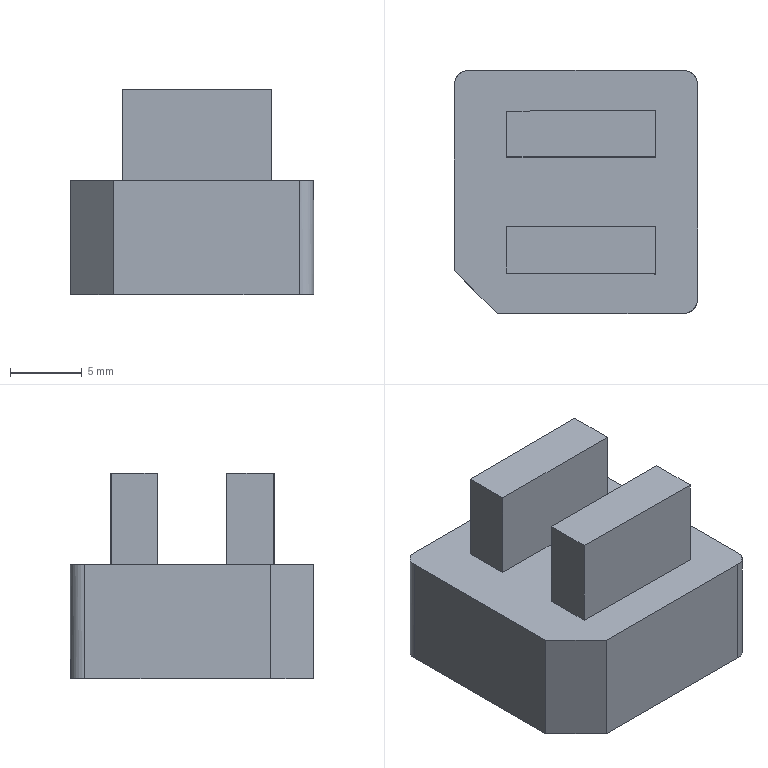NC program | PowerMill | posted with a generic post | part box 17 x 17 x 14.396 mm
Lines 7229 to 8093 of 69084:
N7326 M6
N7327 S18000 M03
N7328 G00 G90 X0.0 Y0.0
N7329 G43 Z10.796 H10
N7330
N7331 G05 P10000 R8
N7332 X6.5722 Y-7.4268
N7333 Z0.918
N7334 G01 Z-0.282 F1200.0
N7335 X6.5582 Y-7.3853 F2000.0
N7336 X6.5405 Y-7.3453
N7337 X6.5192 Y-7.3071
N7338 X6.4946 Y-7.2709
N7339 X6.4667 Y-7.2372
N7340 X6.4359 Y-7.2061
N7341 X6.4024 Y-7.178
N7342 X6.3664 Y-7.153
N7343 X6.3284 Y-7.1314
N7344 X6.2885 Y-7.1134
N7345 X6.2472 Y-7.0991
N7346 X6.2047 Y-7.0886
N7347 X6.1614 Y-7.082
N7348 X6.1178 Y-7.0793
N7349 X6.074 Y-7.0807
N7350 X6.0306 Y-7.086
N7351 X5.9879 Y-7.0953
N7352 X5.9783 Y-7.0979
N7353 X5.9106 Y-7.1174
N7354 X5.8358 Y-7.1349
N7355 X5.7731 Y-7.1469
N7356 X5.7091 Y-7.1555
N7357 X5.6389 Y-7.1612
N7358 X5.5591 Y-7.1639
N7359 X5.4625
N7360 X3.8431 Y-7.1555
N7361 X2.0292 Y-7.1459
N7362 X-1.5322 Y-7.1273
N7363 X-3.5989 Y-7.1165
N7364 X-4.5402 Y-7.1116
N7365 X-4.8986 Y-7.109
N7366 X-4.972 Y-7.1064
N7367 X-5.0454 Y-7.0998
N7368 X-5.1187 Y-7.0892
N7369 X-5.1917 Y-7.0746
N7370 X-5.2643 Y-7.0561
N7371 X-5.3362 Y-7.0336
N7372 X-5.4072 Y-7.0072
N7373 X-5.4764 Y-6.9773
N7374 X-5.544 Y-6.9437
N7375 X-5.6097 Y-6.9066
N7376 X-5.6733 Y-6.866
N7377 X-5.7347 Y-6.8222
N7378 X-5.7937 Y-6.7752
N7379 X-5.8502 Y-6.7251
N7380 X-5.9039 Y-6.6721
N7381 X-5.9547 Y-6.6163
N7382 X-6.0024 Y-6.5579
N7383 X-6.0471 Y-6.4971
N7384 X-6.0884 Y-6.434
N7385 X-6.1264 Y-6.3688
N7386 X-6.1608 Y-6.3016
N7387 X-6.1916 Y-6.2329
N7388 X-6.219 Y-6.1623
N7389 X-6.2424 Y-6.0908
N7390 X-6.2619 Y-6.0185
N7391 X-6.2774 Y-5.9457
N7392 X-6.289 Y-5.8725
N7393 X-6.2966 Y-5.7992
N7394 X-6.3002 Y-5.7258
N7395 X-6.3005 Y-5.6523
N7396 X-6.3012 Y-4.2054
N7397 Y-3.3524
N7398 X-6.3017 Y-2.6994
N7399 X-6.3024 Y-2.4993
N7400 X-6.3011 Y-2.4058
N7401 X-6.2965 Y-2.3214
N7402 X-6.2887 Y-2.2438
N7403 X-6.2779 Y-2.1715
N7404 X-6.264 Y-2.1038
N7405 X-6.2465 Y-2.0368
N7406 X-6.2239 Y-1.9652
N7407 X-6.1974 Y-1.8947
N7408 X-6.1672 Y-1.8256
N7409 X-6.1333 Y-1.758
N7410 X-6.0959 Y-1.6922
N7411 X-6.0549 Y-1.6284
N7412 X-6.0109 Y-1.5671
N7413 X-5.9638 Y-1.5084
N7414 X-5.9137 Y-1.4522
N7415 X-5.8606 Y-1.3987
N7416 X-5.8048 Y-1.3481
N7417 X-5.7463 Y-1.3005
N7418 X-5.6855 Y-1.2561
N7419 X-5.6224 Y-1.215
N7420 X-5.5572 Y-1.1773
N7421 X-5.4901 Y-1.1432
N7422 X-5.4214 Y-1.1126
N7423 X-5.3656 Y-1.0909
N7424 X-5.31 Y-1.0716
N7425 X-5.2537 Y-1.0546
N7426 X-5.1954 Y-1.0398
N7427 X-5.134 Y-1.0273
N7428 X-5.0677 Y-1.0172
N7429 X-4.9943 Y-1.0097
N7430 X-4.9128 Y-1.0052
N7431 X-4.8359 Y-1.0034
N7432 X-4.7635 Y-1.0031
N7433 X-4.6941 Y-1.0033
N7434 X-4.6232 Y-1.0036
N7435 X-4.0059 Y-1.0045
N7436 X-3.399 Y-1.0041
N7437 X3.1113
N7438 X4.6304 Y-1.0037
N7439 X5.4985 Y-1.0031
N7440 X5.5826 Y-1.0047
N7441 X5.6636 Y-1.0098
N7442 X5.7417 Y-1.0183
N7443 X5.8171 Y-1.0304
N7444 X5.8901 Y-1.046
N7445 X5.9609 Y-1.0651
N7446 X6.0297 Y-1.0877
N7447 X6.0967 Y-1.1137
N7448 X6.1625 Y-1.1433
N7449 X6.23 Y-1.1779
N7450 X6.2955 Y-1.2159
N7451 X6.3588 Y-1.2573
N7452 X6.4199 Y-1.302
N7453 X6.4785 Y-1.3499
N7454 X6.5334 Y-1.3996
N7455 X6.5866 Y-1.4532
N7456 X6.6367 Y-1.5093
N7457 X6.6836 Y-1.5678
N7458 X6.727 Y-1.6283
N7459 X6.767 Y-1.6908
N7460 X6.8034 Y-1.7551
N7461 X6.8362 Y-1.821
N7462 X6.8679 Y-1.8929
N7463 X6.8946 Y-1.9626
N7464 X6.9166 Y-2.0305
N7465 X6.9341 Y-2.0969
N7466 X6.9464 Y-2.1543
N7467 X6.9565 Y-2.212
N7468 X6.9642 Y-2.2701
N7469 X6.9696 Y-2.3309
N7470 X6.9729 Y-2.4057
N7471 X6.9738 Y-2.4747
N7472 X6.9737 Y-2.5336
N7473 X6.9735 Y-2.5924
N7474 X6.9734 Y-2.6511
N7475 X6.9731 Y-3.8243
N7476 X6.973 Y-5.0696
N7477 X6.9739 Y-5.6984
N7478 X6.9723 Y-5.7835
N7479 X6.967 Y-5.8646
N7480 X6.9582 Y-5.942
N7481 X6.946 Y-6.0161
N7482 X6.9304 Y-6.0871
N7483 X6.9116 Y-6.1553
N7484 X6.8892 Y-6.2216
N7485 X6.8608 Y-6.2937
N7486 X6.8291 Y-6.3634
N7487 X6.7942 Y-6.4306
N7488 X6.7562 Y-6.4953
N7489 X6.7152 Y-6.5573
N7490 X6.671 Y-6.6169
N7491 X6.623 Y-6.6751
N7492 X6.5719 Y-6.7306
N7493 X6.518 Y-6.7834
N7494 X6.4613 Y-6.8333
N7495 X6.4021 Y-6.8802
N7496 X6.3405 Y-6.9238
N7497 X6.2767 Y-6.9641
N7498 X6.2109 Y-7.0009
N7499 X6.1433 Y-7.0342
N7500 X6.074 Y-7.0639
N7501 X6.0032 Y-7.0898
N7502 X5.9783 Y-7.0979
N7503 X5.9211 Y-7.114
N7504 X5.8523 Y-7.1314 Z-0.2821
N7505 X5.794 Y-7.143
N7506 X5.7224 Y-7.1532 Z-0.2822
N7507 X5.6471 Y-7.1601
N7508 X5.5652 Y-7.1636 Z-0.2823
N7509 X5.4742 Y-7.164 Z-0.2824
N7510 X3.8613 Y-7.1556 Z-0.2837
N7511 X2.0473 Y-7.146 Z-0.2852
N7512 X-1.5144 Y-7.1274 Z-0.2881
N7513 X-3.5989 Y-7.1165 Z-0.2898
N7514 X-4.5388 Y-7.1116 Z-0.2906
N7515 X-4.8986 Y-7.109 Z-0.2909
N7516 X-4.972 Y-7.1064 Z-0.291
N7517 X-5.0454 Y-7.0998
N7518 X-5.1187 Y-7.0892 Z-0.2911
N7519 X-5.1917 Y-7.0746 Z-0.2912
N7520 X-5.2643 Y-7.0561
N7521 X-5.3362 Y-7.0336 Z-0.2913
N7522 X-5.4073 Y-7.0072
N7523 X-5.4764 Y-6.9773 Z-0.2914
N7524 X-5.544 Y-6.9437 Z-0.2915
N7525 X-5.6097 Y-6.9066
N7526 X-5.6734 Y-6.866 Z-0.2916
N7527 X-5.7348 Y-6.8222 Z-0.2917
N7528 X-5.7938 Y-6.7751
N7529 X-5.8502 Y-6.725 Z-0.2918
N7530 X-5.9039 Y-6.672
N7531 X-5.9547 Y-6.6163 Z-0.2919
N7532 X-6.0025 Y-6.5579 Z-0.292
N7533 X-6.0471 Y-6.497
N7534 X-6.0885 Y-6.4339 Z-0.2921
N7535 X-6.1264 Y-6.3687 Z-0.2922
N7536 X-6.1609 Y-6.3016
N7537 X-6.1917 Y-6.2329 Z-0.2923
N7538 X-6.219 Y-6.1623
N7539 X-6.2424 Y-6.0907 Z-0.2924
N7540 X-6.2619 Y-6.0185 Z-0.2925
N7541 X-6.2775 Y-5.9456
N7542 X-6.289 Y-5.8724 Z-0.2926
N7543 X-6.2966 Y-5.7991
N7544 X-6.3002 Y-5.7258 Z-0.2927
N7545 X-6.3005 Y-5.6523 Z-0.2928
N7546 X-6.3012 Y-4.1928 Z-0.294
N7547 Y-3.3325 Z-0.2947
N7548 X-6.3018 Y-2.6011 Z-0.2953
N7549 X-6.3022 Y-2.4722 Z-0.2954
N7550 X-6.301 Y-2.3964
N7551 X-6.2967 Y-2.3205 Z-0.2955
N7552 X-6.2889 Y-2.2449 Z-0.2956
N7553 X-6.2774 Y-2.1708
N7554 X-6.2623 Y-2.099 Z-0.2957
N7555 X-6.2439 Y-2.0295 Z-0.2958
N7556 X-6.2221 Y-1.9608
N7557 X-6.1958 Y-1.891 Z-0.2959
N7558 X-6.1657 Y-1.8224
N7559 X-6.132 Y-1.7554 Z-0.296
N7560 X-6.0946 Y-1.6901 Z-0.2961
N7561 X-6.0537 Y-1.6266
N7562 X-6.0093 Y-1.5652 Z-0.2962
N7563 X-5.9617 Y-1.506
N7564 X-5.9114 Y-1.4499 Z-0.2963
N7565 X-5.8582 Y-1.3965 Z-0.2964
N7566 X-5.8022 Y-1.346
N7567 X-5.7437 Y-1.2985 Z-0.2965
N7568 X-5.6827 Y-1.2542 Z-0.2966
N7569 X-5.6195 Y-1.2133
N7570 X-5.5543 Y-1.1757 Z-0.2967
N7571 X-5.4865 Y-1.1413
N7572 X-5.4174 Y-1.1106 Z-0.2968
N7573 X-5.3472 Y-1.0837 Z-0.2969
N7574 X-5.276 Y-1.0608
N7575 X-5.2042 Y-1.0418 Z-0.297
N7576 X-5.132 Y-1.0268
N7577 X-5.0594 Y-1.0157 Z-0.2971
N7578 X-4.9868 Y-1.0087 Z-0.2972
N7579 X-4.9142 Y-1.0056
N7580 X-4.8415 Y-1.0053 Z-0.2973
N7581 X-3.8933 Y-1.0042 Z-0.2981
N7582 X-2.316 Y-1.0041 Z-0.2994
N7583 X3.5448 Y-1.0039 Z-0.3042
N7584 X5.2855 Y-1.0033 Z-0.3056
N7585 X5.4985 Y-1.003 Z-0.3058
N7586 X5.5827 Y-1.0046 Z-0.3059
N7587 X5.6637 Y-1.0097
N7588 X5.7419 Y-1.0183 Z-0.306
N7589 X5.8173 Y-1.0304 Z-0.3061
N7590 X5.8903 Y-1.046
N7591 X5.961 Y-1.0651 Z-0.3062
N7592 X6.0297 Y-1.0876
N7593 X6.0966 Y-1.1136 Z-0.3063
N7594 X6.1624 Y-1.1432 Z-0.3064
N7595 X6.2299 Y-1.1778
N7596 X6.2954 Y-1.2158 Z-0.3065
N7597 X6.3588 Y-1.2573 Z-0.3066
N7598 X6.4198 Y-1.3019
N7599 X6.4783 Y-1.3497 Z-0.3067
N7600 X6.5343 Y-1.4006
N7601 X6.5874 Y-1.4543 Z-0.3068
N7602 X6.6375 Y-1.5104 Z-0.3069
N7603 X6.6845 Y-1.5692
N7604 X6.7283 Y-1.6304 Z-0.307
N7605 X6.7689 Y-1.6939 Z-0.3071
N7606 X6.8061 Y-1.7595
N7607 X6.8397 Y-1.827 Z-0.3072
N7608 X6.8698 Y-1.8962
N7609 X6.8964 Y-1.967 Z-0.3073
N7610 X6.9188 Y-2.0366 Z-0.3074
N7611 X6.9364 Y-2.1032
N7612 X6.9495 Y-2.1672 Z-0.3075
N7613 X6.9552 Y-2.204
N7614 X6.9606 Y-2.2409
N7615 X6.9661 Y-2.2778 Z-0.3076
N7616 X6.9703 Y-2.3149
N7617 X6.9722 Y-2.3521
N7618 X6.9728 Y-2.3893 Z-0.3077
N7619 X6.9729 Y-2.4266
N7620 X6.9732 Y-2.8429 Z-0.308
N7621 X6.9733 Y-4.3499 Z-0.3093
N7622 X6.9741 Y-5.6983 Z-0.3104
N7623 X6.9724 Y-5.7818
N7624 X6.9671 Y-5.8623 Z-0.3105
N7625 X6.9582 Y-5.94 Z-0.3106
N7626 X6.9457 Y-6.0153
N7627 X6.9297 Y-6.0882 Z-0.3107
N7628 X6.9102 Y-6.1589 Z-0.3108
N7629 X6.8872 Y-6.2277
N7630 X6.8607 Y-6.2947 Z-0.3109
N7631 X6.8306 Y-6.3606
N7632 X6.7956 Y-6.4281 Z-0.311
N7633 X6.7571 Y-6.4935 Z-0.3111
N7634 X6.7154 Y-6.5567
N7635 X6.6704 Y-6.6174 Z-0.3112
N7636 X6.6224 Y-6.6756 Z-0.3113
N7637 X6.5714 Y-6.7311
N7638 X6.5176 Y-6.7839 Z-0.3114
N7639 X6.461 Y-6.8337
N7640 X6.4018 Y-6.8804 Z-0.3115
N7641 X6.3403 Y-6.924 Z-0.3116
N7642 X6.2765 Y-6.9643
N7643 X6.2106 Y-7.0011 Z-0.3117
N7644 X6.143 Y-7.0343 Z-0.3118
N7645 X6.0737 Y-7.064
N7646 X6.0029 Y-7.0899 Z-0.3119
N7647 X5.9783 Y-7.0979
N7648 X5.9211 Y-7.114
N7649 X5.8523 Y-7.1314 Z-0.312
N7650 X5.794 Y-7.143 Z-0.3121
N7651 X5.7224 Y-7.1532
N7652 X5.6471 Y-7.1601 Z-0.3122
N7653 X5.5652 Y-7.1636
N7654 X5.4742 Y-7.164 Z-0.3123
N7655 X3.8613 Y-7.1556 Z-0.3136
N7656 X2.0473 Y-7.146 Z-0.3151
N7657 X-1.5144 Y-7.1274 Z-0.3181
N7658 X-3.5989 Y-7.1165 Z-0.3198
N7659 X-4.5388 Y-7.1116 Z-0.3206
N7660 X-4.8986 Y-7.109 Z-0.3209
N7661 X-4.972 Y-7.1064
N7662 X-5.0454 Y-7.0998 Z-0.321
N7663 X-5.1187 Y-7.0892
N7664 X-5.1917 Y-7.0746 Z-0.3211
N7665 X-5.2643 Y-7.0561 Z-0.3212
N7666 X-5.3362 Y-7.0336
N7667 X-5.4073 Y-7.0072 Z-0.3213
N7668 X-5.4764 Y-6.9773
N7669 X-5.544 Y-6.9437 Z-0.3214
N7670 X-5.6097 Y-6.9066 Z-0.3215
N7671 X-5.6734 Y-6.866
N7672 X-5.7348 Y-6.8222 Z-0.3216
N7673 X-5.7938 Y-6.7751 Z-0.3217
N7674 X-5.8502 Y-6.725
N7675 X-5.9039 Y-6.672 Z-0.3218
N7676 X-5.9547 Y-6.6163
N7677 X-6.0025 Y-6.5579 Z-0.3219
N7678 X-6.0471 Y-6.497 Z-0.322
N7679 X-6.0885 Y-6.4339
N7680 X-6.1264 Y-6.3687 Z-0.3221
N7681 X-6.1609 Y-6.3016 Z-0.3222
N7682 X-6.1917 Y-6.2329
N7683 X-6.219 Y-6.1623 Z-0.3223
N7684 X-6.2424 Y-6.0907
N7685 X-6.2619 Y-6.0185 Z-0.3224
N7686 X-6.2775 Y-5.9456 Z-0.3225
N7687 X-6.289 Y-5.8724
N7688 X-6.2966 Y-5.7991 Z-0.3226
N7689 X-6.3002 Y-5.7258
N7690 X-6.3005 Y-5.6523 Z-0.3227
N7691 X-6.3012 Y-4.1928 Z-0.3239
N7692 Y-3.3325 Z-0.3246
N7693 X-6.3018 Y-2.6011 Z-0.3252
N7694 X-6.3022 Y-2.4722 Z-0.3253
N7695 X-6.301 Y-2.3964 Z-0.3254
N7696 X-6.2967 Y-2.3205 Z-0.3255
N7697 X-6.2889 Y-2.2449
N7698 X-6.2774 Y-2.1708 Z-0.3256
N7699 X-6.2623 Y-2.099
N7700 X-6.2439 Y-2.0295 Z-0.3257
N7701 X-6.2221 Y-1.9608 Z-0.3258
N7702 X-6.1958 Y-1.891
N7703 X-6.1657 Y-1.8224 Z-0.3259
N7704 X-6.132 Y-1.7554
N7705 X-6.0946 Y-1.6901 Z-0.326
N7706 X-6.0537 Y-1.6266 Z-0.3261
N7707 X-6.0093 Y-1.5652
N7708 X-5.9617 Y-1.506 Z-0.3262
N7709 X-5.9114 Y-1.4499
N7710 X-5.8582 Y-1.3965 Z-0.3263
N7711 X-5.8022 Y-1.346 Z-0.3264
N7712 X-5.7437 Y-1.2985
N7713 X-5.6827 Y-1.2542 Z-0.3265
N7714 X-5.6195 Y-1.2133 Z-0.3266
N7715 X-5.5543 Y-1.1757
N7716 X-5.4865 Y-1.1413 Z-0.3267
N7717 X-5.4174 Y-1.1106
N7718 X-5.3472 Y-1.0837 Z-0.3268
N7719 X-5.276 Y-1.0608 Z-0.3269
N7720 X-5.2042 Y-1.0418
N7721 X-5.132 Y-1.0268 Z-0.327
N7722 X-5.0594 Y-1.0157 Z-0.3271
N7723 X-4.9868 Y-1.0087
N7724 X-4.9142 Y-1.0056 Z-0.3272
N7725 X-4.8415 Y-1.0053
N7726 X-3.8933 Y-1.0042 Z-0.328
N7727 X-2.316 Y-1.0041 Z-0.3293
N7728 X3.5448 Y-1.0039 Z-0.3341
N7729 X5.2855 Y-1.0033 Z-0.3356
N7730 X5.4985 Y-1.003 Z-0.3357
N7731 X5.5827 Y-1.0046 Z-0.3358
N7732 X5.6637 Y-1.0097 Z-0.3359
N7733 X5.7419 Y-1.0183
N7734 X5.8173 Y-1.0304 Z-0.336
N7735 X5.8903 Y-1.046 Z-0.3361
N7736 X5.961 Y-1.0651
N7737 X6.0297 Y-1.0876 Z-0.3362
N7738 X6.0966 Y-1.1136
N7739 X6.1624 Y-1.1432 Z-0.3363
N7740 X6.2299 Y-1.1778 Z-0.3364
N7741 X6.2954 Y-1.2158
N7742 X6.3588 Y-1.2573 Z-0.3365
N7743 X6.4198 Y-1.3019 Z-0.3366
N7744 X6.4783 Y-1.3497
N7745 X6.5343 Y-1.4006 Z-0.3367
N7746 X6.5874 Y-1.4543
N7747 X6.6375 Y-1.5104 Z-0.3368
N7748 X6.6845 Y-1.5692 Z-0.3369
N7749 X6.7283 Y-1.6304
N7750 X6.7689 Y-1.6939 Z-0.337
N7751 X6.8061 Y-1.7595 Z-0.3371
N7752 X6.8397 Y-1.827
N7753 X6.8698 Y-1.8962 Z-0.3372
N7754 X6.8964 Y-1.967
N7755 X6.9188 Y-2.0366 Z-0.3373
N7756 X6.9364 Y-2.1032 Z-0.3374
N7757 X6.9495 Y-2.1672
N7758 X6.9552 Y-2.204
N7759 X6.9606 Y-2.2409 Z-0.3375
N7760 X6.9661 Y-2.2778
N7761 X6.9703 Y-2.3149
N7762 X6.9722 Y-2.3521 Z-0.3376
N7763 X6.9728 Y-2.3893
N7764 X6.9729 Y-2.4266
N7765 X6.9732 Y-2.8429 Z-0.338
N7766 X6.9733 Y-4.3499 Z-0.3392
N7767 X6.9741 Y-5.6983 Z-0.3403
N7768 X6.9724 Y-5.7818 Z-0.3404
N7769 X6.9671 Y-5.8623 Z-0.3405
N7770 X6.9582 Y-5.94
N7771 X6.9457 Y-6.0153 Z-0.3406
N7772 X6.9297 Y-6.0882
N7773 X6.9102 Y-6.1589 Z-0.3407
N7774 X6.8872 Y-6.2277 Z-0.3408
N7775 X6.8607 Y-6.2947
N7776 X6.8306 Y-6.3606 Z-0.3409
N7777 X6.7956 Y-6.4281
N7778 X6.7571 Y-6.4935 Z-0.341
N7779 X6.7154 Y-6.5567 Z-0.3411
N7780 X6.6704 Y-6.6174
N7781 X6.6224 Y-6.6756 Z-0.3412
N7782 X6.5714 Y-6.7311 Z-0.3413
N7783 X6.5176 Y-6.7839
N7784 X6.461 Y-6.8337 Z-0.3414
N7785 X6.4018 Y-6.8804
N7786 X6.3403 Y-6.924 Z-0.3415
N7787 X6.2765 Y-6.9643 Z-0.3416
N7788 X6.2106 Y-7.0011
N7789 X6.143 Y-7.0343 Z-0.3417
N7790 X6.0737 Y-7.064 Z-0.3418
N7791 X6.0029 Y-7.0899
N7792 X5.9783 Y-7.0979
N7793 X5.9211 Y-7.114 Z-0.3419
N7794 X5.8523 Y-7.1314
N7795 X5.794 Y-7.143 Z-0.342
N7796 X5.7224 Y-7.1532 Z-0.3421
N7797 X5.6471 Y-7.1601
N7798 X5.5652 Y-7.1636 Z-0.3422
N7799 X5.4742 Y-7.164 Z-0.3423
N7800 X3.8613 Y-7.1556 Z-0.3436
N7801 X2.0473 Y-7.146 Z-0.3451
N7802 X-1.5144 Y-7.1274 Z-0.348
N7803 X-3.5989 Y-7.1165 Z-0.3497
N7804 X-4.5388 Y-7.1116 Z-0.3505
N7805 X-4.8986 Y-7.109 Z-0.3508
N7806 X-4.972 Y-7.1064 Z-0.3509
N7807 X-5.0454 Y-7.0998
N7808 X-5.1187 Y-7.0892 Z-0.351
N7809 X-5.1917 Y-7.0746
N7810 X-5.2643 Y-7.0561 Z-0.3511
N7811 X-5.3362 Y-7.0336 Z-0.3512
N7812 X-5.4073 Y-7.0072
N7813 X-5.4764 Y-6.9773 Z-0.3513
N7814 X-5.544 Y-6.9437 Z-0.3514
N7815 X-5.6097 Y-6.9066
N7816 X-5.6734 Y-6.866 Z-0.3515
N7817 X-5.7348 Y-6.8222
N7818 X-5.7938 Y-6.7751 Z-0.3516
N7819 X-5.8502 Y-6.725 Z-0.3517
N7820 X-5.9039 Y-6.672
N7821 X-5.9547 Y-6.6163 Z-0.3518
N7822 X-6.0025 Y-6.5579
N7823 X-6.0471 Y-6.497 Z-0.3519
N7824 X-6.0885 Y-6.4339 Z-0.352
N7825 X-6.1264 Y-6.3687
N7826 X-6.1609 Y-6.3016 Z-0.3521
N7827 X-6.1917 Y-6.2329 Z-0.3522
N7828 X-6.219 Y-6.1623
N7829 X-6.2424 Y-6.0907 Z-0.3523
N7830 X-6.2619 Y-6.0185
N7831 X-6.2775 Y-5.9456 Z-0.3524
N7832 X-6.289 Y-5.8724 Z-0.3525
N7833 X-6.2966 Y-5.7991
N7834 X-6.3002 Y-5.7258 Z-0.3526
N7835 X-6.3005 Y-5.6523
N7836 X-6.3012 Y-4.1928 Z-0.3539
N7837 Y-3.3325 Z-0.3546
N7838 X-6.3018 Y-2.6011 Z-0.3552
N7839 X-6.3022 Y-2.4722 Z-0.3553
N7840 X-6.301 Y-2.3964
N7841 X-6.2967 Y-2.3205 Z-0.3554
N7842 X-6.2889 Y-2.2449 Z-0.3555
N7843 X-6.2774 Y-2.1708
N7844 X-6.2623 Y-2.099 Z-0.3556
N7845 X-6.2439 Y-2.0295
N7846 X-6.2221 Y-1.9608 Z-0.3557
N7847 X-6.1958 Y-1.891 Z-0.3558
N7848 X-6.1657 Y-1.8224
N7849 X-6.132 Y-1.7554 Z-0.3559
N7850 X-6.0946 Y-1.6901
N7851 X-6.0537 Y-1.6266 Z-0.356
N7852 X-6.0093 Y-1.5652 Z-0.3561
N7853 X-5.9617 Y-1.506
N7854 X-5.9114 Y-1.4499 Z-0.3562
N7855 X-5.8582 Y-1.3965 Z-0.3563
N7856 X-5.8022 Y-1.346
N7857 X-5.7437 Y-1.2985 Z-0.3564
N7858 X-5.6827 Y-1.2542
N7859 X-5.6195 Y-1.2133 Z-0.3565
N7860 X-5.5543 Y-1.1757 Z-0.3566
N7861 X-5.4865 Y-1.1413
N7862 X-5.4174 Y-1.1106 Z-0.3567
N7863 X-5.3472 Y-1.0837 Z-0.3568
N7864 X-5.276 Y-1.0608
N7865 X-5.2042 Y-1.0418 Z-0.3569
N7866 X-5.132 Y-1.0268
N7867 X-5.0594 Y-1.0157 Z-0.357
N7868 X-4.9868 Y-1.0087 Z-0.3571
N7869 X-4.9142 Y-1.0056
N7870 X-4.8415 Y-1.0053 Z-0.3572
N7871 X-3.8933 Y-1.0042 Z-0.358
N7872 X-2.316 Y-1.0041 Z-0.3593
N7873 X3.5448 Y-1.0039 Z-0.3641
N7874 X5.2853 Y-1.0033 Z-0.3655
N7875 X5.4985 Y-1.003 Z-0.3657
N7876 X5.5825 Y-1.0046 Z-0.3658
N7877 X5.6635 Y-1.0097
N7878 X5.7416 Y-1.0182 Z-0.3659
N7879 X5.817 Y-1.0303 Z-0.366
N7880 X5.89 Y-1.0459
N7881 X5.9607 Y-1.065 Z-0.3661
N7882 X6.0295 Y-1.0875
N7883 X6.0964 Y-1.1136 Z-0.3662
N7884 X6.1623 Y-1.1432 Z-0.3663
N7885 X6.2298 Y-1.1777
N7886 X6.2953 Y-1.2158 Z-0.3664
N7887 X6.3586 Y-1.2572
N7888 X6.4197 Y-1.3018 Z-0.3665
N7889 X6.4782 Y-1.3496 Z-0.3666
N7890 X6.5342 Y-1.4005
N7891 X6.5873 Y-1.4542 Z-0.3667
N7892 X6.6374 Y-1.5103
N7893 X6.6844 Y-1.5691 Z-0.3668
N7894 X6.7282 Y-1.6302 Z-0.3669
N7895 X6.7688 Y-1.6937
N7896 X6.806 Y-1.7594 Z-0.367
N7897 X6.8397 Y-1.8269 Z-0.3671
N7898 X6.8697 Y-1.8961
N7899 X6.8964 Y-1.9669 Z-0.3672
N7900 X6.9188 Y-2.0364
N7901 X6.9364 Y-2.103 Z-0.3673
N7902 X6.9494 Y-2.1671 Z-0.3674
N7903 X6.9552 Y-2.2039
N7904 X6.9606 Y-2.2408
N7905 X6.9661 Y-2.2777
N7906 X6.9703 Y-2.3148 Z-0.3675
N7907 X6.9722 Y-2.352
N7908 X6.9728 Y-2.3892
N7909 X6.9729 Y-2.4265 Z-0.3676
N7910 X6.9732 Y-2.8427 Z-0.3679
N7911 X6.9733 Y-4.3498 Z-0.3692
N7912 X6.9741 Y-5.6983 Z-0.3703
N7913 X6.9724 Y-5.7818
N7914 X6.9671 Y-5.8623 Z-0.3704
N7915 X6.9582 Y-5.94 Z-0.3705
N7916 X6.9457 Y-6.0153
N7917 X6.9297 Y-6.0882 Z-0.3706
N7918 X6.9102 Y-6.1589
N7919 X6.8872 Y-6.2277 Z-0.3707
N7920 X6.8607 Y-6.2947 Z-0.3708
N7921 X6.8306 Y-6.3606
N7922 X6.7956 Y-6.4281 Z-0.3709
N7923 X6.7571 Y-6.4935 Z-0.371
N7924 X6.7154 Y-6.5567
N7925 X6.6704 Y-6.6174 Z-0.3711
N7926 X6.6224 Y-6.6756
N7927 X6.5714 Y-6.7311 Z-0.3712
N7928 X6.5176 Y-6.7839 Z-0.3713
N7929 X6.461 Y-6.8337
N7930 X6.4018 Y-6.8804 Z-0.3714
N7931 X6.3403 Y-6.924
N7932 X6.2765 Y-6.9643 Z-0.3715
N7933 X6.2106 Y-7.0011 Z-0.3716
N7934 X6.143 Y-7.0343
N7935 X6.0737 Y-7.064 Z-0.3717
N7936 X6.0029 Y-7.0899 Z-0.3718
N7937 X5.9783 Y-7.0979
N7938 X5.9211 Y-7.114
N7939 X5.8523 Y-7.1314 Z-0.3719
N7940 X5.794 Y-7.143
N7941 X5.7224 Y-7.1532 Z-0.372
N7942 X5.6471 Y-7.1601 Z-0.3721
N7943 X5.5652 Y-7.1636
N7944 X5.4742 Y-7.164 Z-0.3722
N7945 X3.8613 Y-7.1556 Z-0.3735
N7946 X2.0473 Y-7.146 Z-0.375
N7947 X-1.5144 Y-7.1274 Z-0.378
N7948 X-3.5989 Y-7.1165 Z-0.3797
N7949 X-4.5388 Y-7.1116 Z-0.3804
N7950 X-4.8986 Y-7.109 Z-0.3807
N7951 X-4.972 Y-7.1064 Z-0.3808
N7952 X-5.0454 Y-7.0998 Z-0.3809
N7953 X-5.1187 Y-7.0892
N7954 X-5.1917 Y-7.0746 Z-0.381
N7955 X-5.2643 Y-7.0561
N7956 X-5.3362 Y-7.0336 Z-0.3811
N7957 X-5.4073 Y-7.0072 Z-0.3812
N7958 X-5.4764 Y-6.9773
N7959 X-5.544 Y-6.9437 Z-0.3813
N7960 X-5.6097 Y-6.9066 Z-0.3814
N7961 X-5.6734 Y-6.866
N7962 X-5.7348 Y-6.8222 Z-0.3815
N7963 X-5.7938 Y-6.7751
N7964 X-5.8502 Y-6.725 Z-0.3816
N7965 X-5.9039 Y-6.672 Z-0.3817
N7966 X-5.9547 Y-6.6163
N7967 X-6.0025 Y-6.5579 Z-0.3818
N7968 X-6.0471 Y-6.497 Z-0.3819
N7969 X-6.0885 Y-6.4339
N7970 X-6.1264 Y-6.3687 Z-0.382
N7971 X-6.1609 Y-6.3016
N7972 X-6.1917 Y-6.2329 Z-0.3821
N7973 X-6.219 Y-6.1623 Z-0.3822
N7974 X-6.2424 Y-6.0907
N7975 X-6.2619 Y-6.0185 Z-0.3823
N7976 X-6.2775 Y-5.9456
N7977 X-6.289 Y-5.8724 Z-0.3824
N7978 X-6.2966 Y-5.7991 Z-0.3825
N7979 X-6.3002 Y-5.7258
N7980 X-6.3005 Y-5.6523 Z-0.3826
N7981 X-6.3012 Y-4.1928 Z-0.3838
N7982 Y-3.3325 Z-0.3845
N7983 X-6.3018 Y-2.6011 Z-0.3851
N7984 X-6.3022 Y-2.4722 Z-0.3852
N7985 X-6.301 Y-2.3964 Z-0.3853
N7986 X-6.2967 Y-2.3205
N7987 X-6.2889 Y-2.2449 Z-0.3854
N7988 X-6.2774 Y-2.1708 Z-0.3855
N7989 X-6.2623 Y-2.099
N7990 X-6.2439 Y-2.0295 Z-0.3856
N7991 X-6.2221 Y-1.9608
N7992 X-6.1958 Y-1.891 Z-0.3857
N7993 X-6.1657 Y-1.8224 Z-0.3858
N7994 X-6.132 Y-1.7554
N7995 X-6.0946 Y-1.6901 Z-0.3859
N7996 X-6.0537 Y-1.6266
N7997 X-6.0093 Y-1.5652 Z-0.386
N7998 X-5.9617 Y-1.506 Z-0.3861
N7999 X-5.9114 Y-1.4499
N8000 X-5.8582 Y-1.3965 Z-0.3862
N8001 X-5.8022 Y-1.346 Z-0.3863
N8002 X-5.7437 Y-1.2985
N8003 X-5.6827 Y-1.2542 Z-0.3864
N8004 X-5.6195 Y-1.2133
N8005 X-5.5543 Y-1.1757 Z-0.3865
N8006 X-5.4865 Y-1.1413 Z-0.3866
N8007 X-5.4174 Y-1.1106
N8008 X-5.3472 Y-1.0837 Z-0.3867
N8009 X-5.276 Y-1.0608 Z-0.3868
N8010 X-5.2042 Y-1.0418
N8011 X-5.132 Y-1.0268 Z-0.3869
N8012 X-5.0594 Y-1.0157
N8013 X-4.9868 Y-1.0087 Z-0.387
N8014 X-4.9142 Y-1.0056 Z-0.3871
N8015 X-4.8415 Y-1.0053
N8016 X-3.8933 Y-1.0042 Z-0.3879
N8017 X-2.316 Y-1.0041 Z-0.3892
N8018 X3.5448 Y-1.0039 Z-0.394
N8019 X5.2855 Y-1.0033 Z-0.3955
N8020 X5.4985 Y-1.003 Z-0.3956
N8021 X5.5827 Y-1.0046 Z-0.3957
N8022 X5.6637 Y-1.0097 Z-0.3958
N8023 X5.7419 Y-1.0183
N8024 X5.8173 Y-1.0304 Z-0.3959
N8025 X5.8903 Y-1.046 Z-0.396
N8026 X5.961 Y-1.0651
N8027 X6.0297 Y-1.0876 Z-0.3961
N8028 X6.0966 Y-1.1136
N8029 X6.1624 Y-1.1432 Z-0.3962
N8030 X6.2299 Y-1.1778 Z-0.3963
N8031 X6.2954 Y-1.2158
N8032 X6.3588 Y-1.2573 Z-0.3964
N8033 X6.4198 Y-1.3019
N8034 X6.4783 Y-1.3497 Z-0.3965
N8035 X6.5343 Y-1.4006 Z-0.3966
N8036 X6.5874 Y-1.4543
N8037 X6.6375 Y-1.5104 Z-0.3967
N8038 X6.6845 Y-1.5692 Z-0.3968
N8039 X6.7283 Y-1.6304
N8040 X6.7689 Y-1.6939 Z-0.3969
N8041 X6.8061 Y-1.7595
N8042 X6.8397 Y-1.827 Z-0.397
N8043 X6.8698 Y-1.8962 Z-0.3971
N8044 X6.8964 Y-1.967
N8045 X6.9188 Y-2.0366 Z-0.3972
N8046 X6.9364 Y-2.1032
N8047 X6.9495 Y-2.1672 Z-0.3973
N8048 X6.9552 Y-2.204
N8049 X6.9606 Y-2.2409 Z-0.3974
N8050 X6.9661 Y-2.2778
N8051 X6.9703 Y-2.3149
N8052 X6.9722 Y-2.3521 Z-0.3975
N8053 X6.9728 Y-2.3893
N8054 X6.9729 Y-2.4266
N8055 X6.9732 Y-2.8429 Z-0.3979
N8056 X6.9733 Y-4.3499 Z-0.3991
N8057 X6.9741 Y-5.6983 Z-0.4002
N8058 X6.9724 Y-5.7818 Z-0.4003
N8059 X6.9671 Y-5.8623
N8060 X6.9582 Y-5.94 Z-0.4004
N8061 X6.9457 Y-6.0153 Z-0.4005
N8062 X6.9297 Y-6.0882
N8063 X6.9102 Y-6.1589 Z-0.4006
N8064 X6.8872 Y-6.2277 Z-0.4007
N8065 X6.8607 Y-6.2947
N8066 X6.8306 Y-6.3606 Z-0.4008
N8067 X6.7956 Y-6.4281
N8068 X6.7571 Y-6.4935 Z-0.4009
N8069 X6.7154 Y-6.5567 Z-0.401
N8070 X6.6704 Y-6.6174
N8071 X6.6224 Y-6.6756 Z-0.4011
N8072 X6.5714 Y-6.7311
N8073 X6.5176 Y-6.7839 Z-0.4012
N8074 X6.461 Y-6.8337 Z-0.4013
N8075 X6.4018 Y-6.8804
N8076 X6.3403 Y-6.924 Z-0.4014
N8077 X6.2765 Y-6.9643 Z-0.4015
N8078 X6.2106 Y-7.0011
N8079 X6.143 Y-7.0343 Z-0.4016
N8080 X6.0737 Y-7.064
N8081 X6.0029 Y-7.0899 Z-0.4017
N8082 X5.9783 Y-7.0979
N8083 X5.9211 Y-7.114 Z-0.4018
N8084 X5.8523 Y-7.1314
N8085 X5.794 Y-7.143 Z-0.4019
N8086 X5.7224 Y-7.1532
N8087 X5.6471 Y-7.1601 Z-0.402
N8088 X5.5652 Y-7.1636 Z-0.4021
N8089 X5.4742 Y-7.164
N8090 X3.8613 Y-7.1556 Z-0.4035
N8091 X2.0473 Y-7.146 Z-0.405
N8092 X-1.5144 Y-7.1274 Z-0.4079
N8093 X-3.5989 Y-7.1165 Z-0.4096
N8094 X-4.5388 Y-7.1116 Z-0.4104
N8095 X-4.8986 Y-7.109 Z-0.4107
N8096 X-4.972 Y-7.1064
N8097 X-5.0454 Y-7.0998 Z-0.4108
N8098 X-5.1187 Y-7.0892 Z-0.4109
N8099 X-5.1917 Y-7.0746
N8100 X-5.2643 Y-7.0561 Z-0.411
N8101 X-5.3362 Y-7.0336 Z-0.4111
N8102 X-5.4073 Y-7.0072
N8103 X-5.4764 Y-6.9773 Z-0.4112
N8104 X-5.544 Y-6.9437
N8105 X-5.6097 Y-6.9066 Z-0.4113
N8106 X-5.6734 Y-6.866 Z-0.4114
N8107 X-5.7348 Y-6.8222
N8108 X-5.7938 Y-6.7751 Z-0.4115
N8109 X-5.8502 Y-6.725 Z-0.4116
N8110 X-5.9039 Y-6.672
N8111 X-5.9547 Y-6.6163 Z-0.4117
N8112 X-6.0025 Y-6.5579
N8113 X-6.0471 Y-6.497 Z-0.4118
N8114 X-6.0885 Y-6.4339 Z-0.4119
N8115 X-6.1264 Y-6.3687
N8116 X-6.1609 Y-6.3016 Z-0.412
N8117 X-6.1917 Y-6.2329
N8118 X-6.219 Y-6.1623 Z-0.4121
N8119 X-6.2424 Y-6.0907 Z-0.4122
N8120 X-6.2619 Y-6.0185
N8121 X-6.2775 Y-5.9456 Z-0.4123
N8122 X-6.289 Y-5.8724 Z-0.4124
N8123 X-6.2966 Y-5.7991
N8124 X-6.3002 Y-5.7258 Z-0.4125
N8125 X-6.3005 Y-5.6523
N8126 X-6.3012 Y-4.1928 Z-0.4137
N8127 Y-3.3325 Z-0.4144
N8128 X-6.3018 Y-2.6011 Z-0.415
N8129 X-6.3022 Y-2.4722 Z-0.4152
N8130 X-6.301 Y-2.3964
N8131 X-6.2967 Y-2.3205 Z-0.4153
N8132 X-6.2889 Y-2.2449
N8133 X-6.2774 Y-2.1708 Z-0.4154
N8134 X-6.2623 Y-2.099 Z-0.4155
N8135 X-6.2439 Y-2.0295
N8136 X-6.2221 Y-1.9608 Z-0.4156
N8137 X-6.1958 Y-1.891
N8138 X-6.1657 Y-1.8224 Z-0.4157
N8139 X-6.132 Y-1.7554 Z-0.4158
N8140 X-6.0946 Y-1.6901
N8141 X-6.0537 Y-1.6266 Z-0.4159
N8142 X-6.0093 Y-1.5652 Z-0.416
N8143 X-5.9617 Y-1.506
N8144 X-5.9114 Y-1.4499 Z-0.4161
N8145 X-5.8582 Y-1.3965
N8146 X-5.8022 Y-1.346 Z-0.4162
N8147 X-5.7437 Y-1.2985 Z-0.4163
N8148 X-5.6827 Y-1.2542
N8149 X-5.6195 Y-1.2133 Z-0.4164
N8150 X-5.5543 Y-1.1757 Z-0.4165
N8151 X-5.4865 Y-1.1413
N8152 X-5.4174 Y-1.1106 Z-0.4166
N8153 X-5.3472 Y-1.0837
N8154 X-5.276 Y-1.0608 Z-0.4167
N8155 X-5.2042 Y-1.0418 Z-0.4168
N8156 X-5.132 Y-1.0268
N8157 X-5.0594 Y-1.0157 Z-0.4169
N8158 X-4.9868 Y-1.0087
N8159 X-4.9142 Y-1.0056 Z-0.417
N8160 X-4.8415 Y-1.0053 Z-0.4171
N8161 X-3.8933 Y-1.0042 Z-0.4178
N8162 X-2.316 Y-1.0041 Z-0.4191
N8163 X3.5448 Y-1.0039 Z-0.424
N8164 X5.2855 Y-1.0033 Z-0.4254
N8165 X5.4985 Y-1.003 Z-0.4256
N8166 X5.5827 Y-1.0046
N8167 X5.6637 Y-1.0097 Z-0.4257
N8168 X5.7419 Y-1.0183 Z-0.4258
N8169 X5.8173 Y-1.0304
N8170 X5.8903 Y-1.046 Z-0.4259
N8171 X5.961 Y-1.0651 Z-0.426
N8172 X6.0297 Y-1.0876
N8173 X6.0966 Y-1.1136 Z-0.4261
N8174 X6.1624 Y-1.1432
N8175 X6.2299 Y-1.1778 Z-0.4262
N8176 X6.2954 Y-1.2158 Z-0.4263
N8177 X6.3588 Y-1.2573
N8178 X6.4198 Y-1.3019 Z-0.4264
N8179 X6.4783 Y-1.3497
N8180 X6.5343 Y-1.4006 Z-0.4265
N8181 X6.5874 Y-1.4543 Z-0.4266
N8182 X6.6375 Y-1.5104
N8183 X6.6845 Y-1.5692 Z-0.4267
N8184 X6.7283 Y-1.6304 Z-0.4268
N8185 X6.7689 Y-1.6939
N8186 X6.8061 Y-1.7595 Z-0.4269
N8187 X6.8397 Y-1.827
N8188 X6.8698 Y-1.8962 Z-0.427
N8189 X6.8964 Y-1.967 Z-0.4271
N8190 X6.9188 Y-2.0366